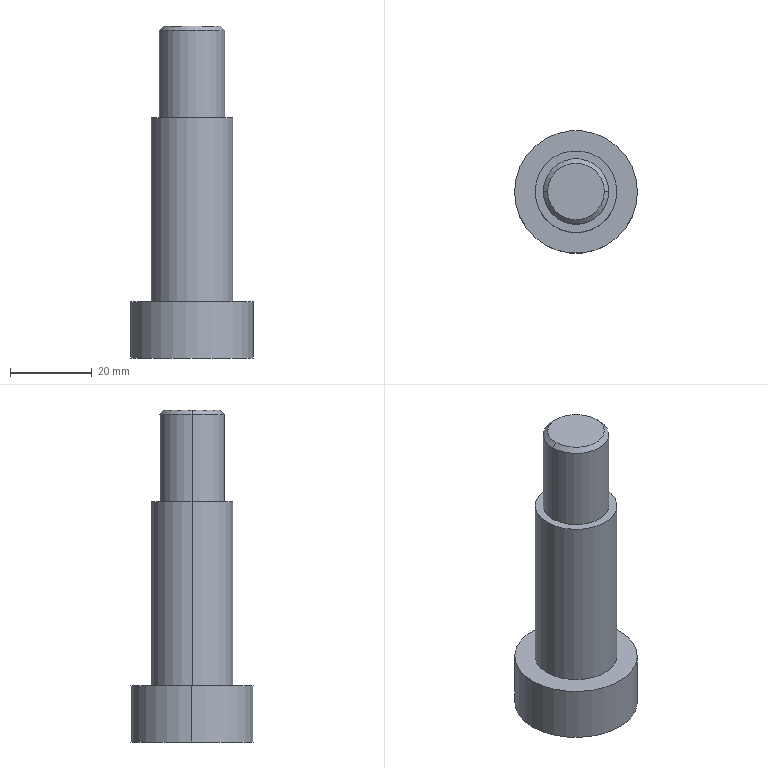Part | SolidWorks | features BaseBody 1 | 1 solid | 12 faces | box 30 x 30 x 81.15 mm | volume 28332 mm3 | cylinder 6 | plane 4 | cone 2 | commonest cylinder face diameters 16 x2 20 x2 30 x2
STEP:
#1=CARTESIAN_POINT('',(-6.918,0.,0.));
#2=VERTEX_POINT('',#1);
#3=CARTESIAN_POINT('',(6.918,0.,0.));
#4=VERTEX_POINT('',#3);
#5=CARTESIAN_POINT('',(0.,0.,0.));
#6=DIRECTION('',(0.,0.,-1.));
#7=DIRECTION('',(-1.,0.,0.));
#8=AXIS2_PLACEMENT_3D('',#5,#6,#7);
#9=CIRCLE('',#8,6.918);
#10=EDGE_CURVE('',#2,#4,#9,.T.);
#11=ORIENTED_EDGE('',*,*,#10,.T.);
#12=CARTESIAN_POINT('',(8.,0.,-1.082));
#13=VERTEX_POINT('',#12);
#14=CARTESIAN_POINT('',(6.918,0.,0.));
#15=DIRECTION('',(0.7071,0.,-0.7071));
#16=VECTOR('',#15,1000.);
#17=LINE('',#14,#16);
#18=EDGE_CURVE('',#4,#13,#17,.T.);
#19=ORIENTED_EDGE('',*,*,#18,.T.);
#20=CARTESIAN_POINT('',(-8.,0.,-1.082));
#21=VERTEX_POINT('',#20);
#22=CARTESIAN_POINT('',(0.,0.,-1.082));
#23=DIRECTION('',(0.,0.,-1.));
#24=DIRECTION('',(-1.,0.,0.));
#25=AXIS2_PLACEMENT_3D('',#22,#23,#24);
#26=CIRCLE('',#25,8.);
#27=EDGE_CURVE('',#21,#13,#26,.T.);
#28=ORIENTED_EDGE('',*,*,#27,.F.);
#29=CARTESIAN_POINT('',(-6.918,0.,0.));
#30=DIRECTION('',(-0.7071,0.,-0.7071));
#31=VECTOR('',#30,1000.);
#32=LINE('',#29,#31);
#33=EDGE_CURVE('',#2,#21,#32,.T.);
#34=ORIENTED_EDGE('',*,*,#33,.F.);
#35=EDGE_LOOP('',(#11,#19,#28,#34));
#36=FACE_OUTER_BOUND('',#35,.T.);
#37=CARTESIAN_POINT('',(0.,0.,0.));
#38=DIRECTION('',(0.,0.,-1.));
#39=DIRECTION('',(-1.,0.,0.));
#40=AXIS2_PLACEMENT_3D('',#37,#38,#39);
#41=CONICAL_SURFACE('',#40,6.918,0.7854);
#42=ADVANCED_FACE('',(#36),#41,.T.);
#43=CARTESIAN_POINT('',(8.,0.,-22.4));
#44=VERTEX_POINT('',#43);
#45=CARTESIAN_POINT('',(-8.,0.,-22.4));
#46=VERTEX_POINT('',#45);
#47=CARTESIAN_POINT('',(0.,0.,-22.4));
#48=DIRECTION('',(0.,0.,1.));
#49=DIRECTION('',(1.,0.,0.));
#50=AXIS2_PLACEMENT_3D('',#47,#48,#49);
#51=CIRCLE('',#50,8.);
#52=EDGE_CURVE('',#44,#46,#51,.T.);
#53=ORIENTED_EDGE('',*,*,#52,.T.);
#54=CARTESIAN_POINT('',(-8.,0.,0.));
#55=DIRECTION('',(0.,0.,1.));
#56=VECTOR('',#55,1000.);
#57=LINE('',#54,#56);
#58=EDGE_CURVE('',#46,#21,#57,.T.);
#59=ORIENTED_EDGE('',*,*,#58,.T.);
#60=ORIENTED_EDGE('',*,*,#27,.T.);
#61=CARTESIAN_POINT('',(8.,0.,0.));
#62=DIRECTION('',(0.,0.,1.));
#63=VECTOR('',#62,1000.);
#64=LINE('',#61,#63);
#65=EDGE_CURVE('',#44,#13,#64,.T.);
#66=ORIENTED_EDGE('',*,*,#65,.F.);
#67=EDGE_LOOP('',(#53,#59,#60,#66));
#68=FACE_OUTER_BOUND('',#67,.T.);
#69=CARTESIAN_POINT('',(0.,0.,0.));
#70=DIRECTION('',(0.,0.,1.));
#71=DIRECTION('',(1.,0.,0.));
#72=AXIS2_PLACEMENT_3D('',#69,#70,#71);
#73=CYLINDRICAL_SURFACE('',#72,8.);
#74=ADVANCED_FACE('',(#68),#73,.T.);
#75=CARTESIAN_POINT('',(10.,0.,-67.4));
#76=VERTEX_POINT('',#75);
#77=CARTESIAN_POINT('',(-10.,0.,-67.4));
#78=VERTEX_POINT('',#77);
#79=CARTESIAN_POINT('',(0.,0.,-67.4));
#80=DIRECTION('',(0.,0.,1.));
#81=DIRECTION('',(1.,0.,0.));
#82=AXIS2_PLACEMENT_3D('',#79,#80,#81);
#83=CIRCLE('',#82,10.);
#84=EDGE_CURVE('',#76,#78,#83,.T.);
#85=ORIENTED_EDGE('',*,*,#84,.T.);
#86=CARTESIAN_POINT('',(-10.,0.,-22.4));
#87=VERTEX_POINT('',#86);
#88=CARTESIAN_POINT('',(-10.,0.,0.));
#89=DIRECTION('',(0.,0.,1.));
#90=VECTOR('',#89,1000.);
#91=LINE('',#88,#90);
#92=EDGE_CURVE('',#78,#87,#91,.T.);
#93=ORIENTED_EDGE('',*,*,#92,.T.);
#94=CARTESIAN_POINT('',(10.,0.,-22.4));
#95=VERTEX_POINT('',#94);
#96=CARTESIAN_POINT('',(0.,0.,-22.4));
#97=DIRECTION('',(0.,0.,1.));
#98=DIRECTION('',(1.,0.,0.));
#99=AXIS2_PLACEMENT_3D('',#96,#97,#98);
#100=CIRCLE('',#99,10.);
#101=EDGE_CURVE('',#95,#87,#100,.T.);
#102=ORIENTED_EDGE('',*,*,#101,.F.);
#103=CARTESIAN_POINT('',(10.,0.,0.));
#104=DIRECTION('',(0.,0.,1.));
#105=VECTOR('',#104,1000.);
#106=LINE('',#103,#105);
#107=EDGE_CURVE('',#76,#95,#106,.T.);
#108=ORIENTED_EDGE('',*,*,#107,.F.);
#109=EDGE_LOOP('',(#85,#93,#102,#108));
#110=FACE_OUTER_BOUND('',#109,.T.);
#111=CARTESIAN_POINT('',(0.,0.,0.));
#112=DIRECTION('',(0.,0.,1.));
#113=DIRECTION('',(1.,0.,0.));
#114=AXIS2_PLACEMENT_3D('',#111,#112,#113);
#115=CYLINDRICAL_SURFACE('',#114,10.);
#116=ADVANCED_FACE('',(#110),#115,.T.);
#117=CARTESIAN_POINT('',(15.,0.,-81.15));
#118=VERTEX_POINT('',#117);
#119=CARTESIAN_POINT('',(-15.,0.,-81.15));
#120=VERTEX_POINT('',#119);
#121=CARTESIAN_POINT('',(0.,0.,-81.15));
#122=DIRECTION('',(0.,0.,1.));
#123=DIRECTION('',(1.,0.,0.));
#124=AXIS2_PLACEMENT_3D('',#121,#122,#123);
#125=CIRCLE('',#124,15.);
#126=EDGE_CURVE('',#118,#120,#125,.T.);
#127=ORIENTED_EDGE('',*,*,#126,.T.);
#128=CARTESIAN_POINT('',(-15.,0.,-67.4));
#129=VERTEX_POINT('',#128);
#130=CARTESIAN_POINT('',(-15.,0.,0.));
#131=DIRECTION('',(0.,0.,1.));
#132=VECTOR('',#131,1000.);
#133=LINE('',#130,#132);
#134=EDGE_CURVE('',#120,#129,#133,.T.);
#135=ORIENTED_EDGE('',*,*,#134,.T.);
#136=CARTESIAN_POINT('',(15.,0.,-67.4));
#137=VERTEX_POINT('',#136);
#138=CARTESIAN_POINT('',(0.,0.,-67.4));
#139=DIRECTION('',(0.,0.,1.));
#140=DIRECTION('',(1.,0.,0.));
#141=AXIS2_PLACEMENT_3D('',#138,#139,#140);
#142=CIRCLE('',#141,15.);
#143=EDGE_CURVE('',#137,#129,#142,.T.);
#144=ORIENTED_EDGE('',*,*,#143,.F.);
#145=CARTESIAN_POINT('',(15.,0.,0.));
#146=DIRECTION('',(0.,0.,1.));
#147=VECTOR('',#146,1000.);
#148=LINE('',#145,#147);
#149=EDGE_CURVE('',#118,#137,#148,.T.);
#150=ORIENTED_EDGE('',*,*,#149,.F.);
#151=EDGE_LOOP('',(#127,#135,#144,#150));
#152=FACE_OUTER_BOUND('',#151,.T.);
#153=CARTESIAN_POINT('',(0.,0.,0.));
#154=DIRECTION('',(0.,0.,1.));
#155=DIRECTION('',(1.,0.,0.));
#156=AXIS2_PLACEMENT_3D('',#153,#154,#155);
#157=CYLINDRICAL_SURFACE('',#156,15.);
#158=ADVANCED_FACE('',(#152),#157,.T.);
#159=ORIENTED_EDGE('',*,*,#10,.F.);
#160=CARTESIAN_POINT('',(0.,0.,0.));
#161=DIRECTION('',(0.,0.,-1.));
#162=DIRECTION('',(-1.,0.,0.));
#163=AXIS2_PLACEMENT_3D('',#160,#161,#162);
#164=CIRCLE('',#163,6.918);
#165=EDGE_CURVE('',#4,#2,#164,.T.);
#166=ORIENTED_EDGE('',*,*,#165,.F.);
#167=EDGE_LOOP('',(#159,#166));
#168=FACE_OUTER_BOUND('',#167,.T.);
#169=CARTESIAN_POINT('',(0.,8.,0.));
#170=DIRECTION('',(0.,0.,-1.));
#171=DIRECTION('',(0.,-1.,0.));
#172=AXIS2_PLACEMENT_3D('',#169,#170,#171);
#173=PLANE('',#172);
#174=ADVANCED_FACE('',(#168),#173,.F.);
#175=ORIENTED_EDGE('',*,*,#52,.F.);
#176=CARTESIAN_POINT('',(0.,0.,-22.4));
#177=DIRECTION('',(0.,0.,1.));
#178=DIRECTION('',(1.,0.,0.));
#179=AXIS2_PLACEMENT_3D('',#176,#177,#178);
#180=CIRCLE('',#179,8.);
#181=EDGE_CURVE('',#46,#44,#180,.T.);
#182=ORIENTED_EDGE('',*,*,#181,.F.);
#183=EDGE_LOOP('',(#175,#182));
#184=FACE_BOUND('',#183,.T.);
#185=ORIENTED_EDGE('',*,*,#101,.T.);
#186=CARTESIAN_POINT('',(0.,0.,-22.4));
#187=DIRECTION('',(0.,0.,1.));
#188=DIRECTION('',(1.,0.,0.));
#189=AXIS2_PLACEMENT_3D('',#186,#187,#188);
#190=CIRCLE('',#189,10.);
#191=EDGE_CURVE('',#87,#95,#190,.T.);
#192=ORIENTED_EDGE('',*,*,#191,.T.);
#193=EDGE_LOOP('',(#185,#192));
#194=FACE_OUTER_BOUND('',#193,.T.);
#195=CARTESIAN_POINT('',(0.,10.,-22.4));
#196=DIRECTION('',(0.,0.,-1.));
#197=DIRECTION('',(0.,-1.,0.));
#198=AXIS2_PLACEMENT_3D('',#195,#196,#197);
#199=PLANE('',#198);
#200=ADVANCED_FACE('',(#184,#194),#199,.F.);
#201=ORIENTED_EDGE('',*,*,#84,.F.);
#202=CARTESIAN_POINT('',(0.,0.,-67.4));
#203=DIRECTION('',(0.,0.,1.));
#204=DIRECTION('',(1.,0.,0.));
#205=AXIS2_PLACEMENT_3D('',#202,#203,#204);
#206=CIRCLE('',#205,10.);
#207=EDGE_CURVE('',#78,#76,#206,.T.);
#208=ORIENTED_EDGE('',*,*,#207,.F.);
#209=EDGE_LOOP('',(#201,#208));
#210=FACE_BOUND('',#209,.T.);
#211=ORIENTED_EDGE('',*,*,#143,.T.);
#212=CARTESIAN_POINT('',(0.,0.,-67.4));
#213=DIRECTION('',(0.,0.,1.));
#214=DIRECTION('',(1.,0.,0.));
#215=AXIS2_PLACEMENT_3D('',#212,#213,#214);
#216=CIRCLE('',#215,15.);
#217=EDGE_CURVE('',#129,#137,#216,.T.);
#218=ORIENTED_EDGE('',*,*,#217,.T.);
#219=EDGE_LOOP('',(#211,#218));
#220=FACE_OUTER_BOUND('',#219,.T.);
#221=CARTESIAN_POINT('',(0.,15.,-67.4));
#222=DIRECTION('',(0.,0.,-1.));
#223=DIRECTION('',(0.,-1.,0.));
#224=AXIS2_PLACEMENT_3D('',#221,#222,#223);
#225=PLANE('',#224);
#226=ADVANCED_FACE('',(#210,#220),#225,.F.);
#227=ORIENTED_EDGE('',*,*,#126,.F.);
#228=CARTESIAN_POINT('',(0.,0.,-81.15));
#229=DIRECTION('',(0.,0.,1.));
#230=DIRECTION('',(1.,0.,0.));
#231=AXIS2_PLACEMENT_3D('',#228,#229,#230);
#232=CIRCLE('',#231,15.);
#233=EDGE_CURVE('',#120,#118,#232,.T.);
#234=ORIENTED_EDGE('',*,*,#233,.F.);
#235=EDGE_LOOP('',(#227,#234));
#236=FACE_OUTER_BOUND('',#235,.T.);
#237=CARTESIAN_POINT('',(0.,0.,-81.15));
#238=DIRECTION('',(0.,0.,1.));
#239=DIRECTION('',(1.,0.,0.));
#240=AXIS2_PLACEMENT_3D('',#237,#238,#239);
#241=PLANE('',#240);
#242=ADVANCED_FACE('',(#236),#241,.F.);
#243=ORIENTED_EDGE('',*,*,#134,.F.);
#244=ORIENTED_EDGE('',*,*,#233,.T.);
#245=ORIENTED_EDGE('',*,*,#149,.T.);
#246=ORIENTED_EDGE('',*,*,#217,.F.);
#247=EDGE_LOOP('',(#243,#244,#245,#246));
#248=FACE_OUTER_BOUND('',#247,.T.);
#249=CARTESIAN_POINT('',(0.,0.,0.));
#250=DIRECTION('',(0.,0.,1.));
#251=DIRECTION('',(1.,0.,0.));
#252=AXIS2_PLACEMENT_3D('',#249,#250,#251);
#253=CYLINDRICAL_SURFACE('',#252,15.);
#254=ADVANCED_FACE('',(#248),#253,.T.);
#255=ORIENTED_EDGE('',*,*,#92,.F.);
#256=ORIENTED_EDGE('',*,*,#207,.T.);
#257=ORIENTED_EDGE('',*,*,#107,.T.);
#258=ORIENTED_EDGE('',*,*,#191,.F.);
#259=EDGE_LOOP('',(#255,#256,#257,#258));
#260=FACE_OUTER_BOUND('',#259,.T.);
#261=CARTESIAN_POINT('',(0.,0.,0.));
#262=DIRECTION('',(0.,0.,1.));
#263=DIRECTION('',(1.,0.,0.));
#264=AXIS2_PLACEMENT_3D('',#261,#262,#263);
#265=CYLINDRICAL_SURFACE('',#264,10.);
#266=ADVANCED_FACE('',(#260),#265,.T.);
#267=ORIENTED_EDGE('',*,*,#58,.F.);
#268=ORIENTED_EDGE('',*,*,#181,.T.);
#269=ORIENTED_EDGE('',*,*,#65,.T.);
#270=CARTESIAN_POINT('',(0.,0.,-1.082));
#271=DIRECTION('',(0.,0.,-1.));
#272=DIRECTION('',(-1.,0.,0.));
#273=AXIS2_PLACEMENT_3D('',#270,#271,#272);
#274=CIRCLE('',#273,8.);
#275=EDGE_CURVE('',#13,#21,#274,.T.);
#276=ORIENTED_EDGE('',*,*,#275,.T.);
#277=EDGE_LOOP('',(#267,#268,#269,#276));
#278=FACE_OUTER_BOUND('',#277,.T.);
#279=CARTESIAN_POINT('',(0.,0.,0.));
#280=DIRECTION('',(0.,0.,1.));
#281=DIRECTION('',(1.,0.,0.));
#282=AXIS2_PLACEMENT_3D('',#279,#280,#281);
#283=CYLINDRICAL_SURFACE('',#282,8.);
#284=ADVANCED_FACE('',(#278),#283,.T.);
#285=ORIENTED_EDGE('',*,*,#18,.F.);
#286=ORIENTED_EDGE('',*,*,#165,.T.);
#287=ORIENTED_EDGE('',*,*,#33,.T.);
#288=ORIENTED_EDGE('',*,*,#275,.F.);
#289=EDGE_LOOP('',(#285,#286,#287,#288));
#290=FACE_OUTER_BOUND('',#289,.T.);
#291=CARTESIAN_POINT('',(0.,0.,0.));
#292=DIRECTION('',(0.,0.,-1.));
#293=DIRECTION('',(-1.,0.,0.));
#294=AXIS2_PLACEMENT_3D('',#291,#292,#293);
#295=CONICAL_SURFACE('',#294,6.918,0.7854);
#296=ADVANCED_FACE('',(#290),#295,.T.);
#297=CLOSED_SHELL('',(#42,#74,#116,#158,#174,#200,#226,#242,#254,#266,#284,#296));
#298=MANIFOLD_SOLID_BREP('',#297);
#299=CARTESIAN_POINT('',(0.,0.,0.));
#300=DIRECTION('',(0.,0.,1.));
#301=DIRECTION('',(1.,0.,0.));
#302=AXIS2_PLACEMENT_3D('',#299,#300,#301);
#303=(LENGTH_UNIT()NAMED_UNIT(*)SI_UNIT(.MILLI.,.METRE.));
#304=UNCERTAINTY_MEASURE_WITH_UNIT(LENGTH_MEASURE(0.00001),#303,'','');
#305=(NAMED_UNIT(*)PLANE_ANGLE_UNIT()SI_UNIT($,.RADIAN.));
#306=(NAMED_UNIT(*)SI_UNIT($,.STERADIAN.)SOLID_ANGLE_UNIT());
#307=(GEOMETRIC_REPRESENTATION_CONTEXT(3)GLOBAL_UNCERTAINTY_ASSIGNED_CONTEXT((#304))GLOBAL_UNIT_ASSIGNED_CONTEXT((#303,#305,#306))REPRESENTATION_CONTEXT('',''));
#308=ADVANCED_BREP_SHAPE_REPRESENTATION('',(#298,#302),#307);